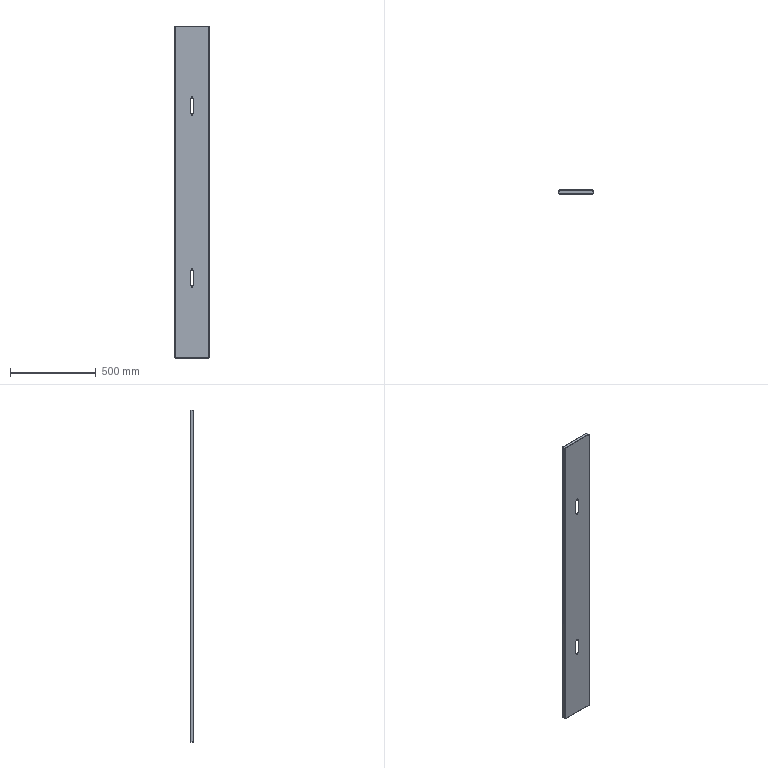Part | STEP file | JBJ-P-1011-07 | 1 solid | 114 faces | box 200 x 20 x 1935 mm | volume 617384 mm3 | plane 58 | cylinder 40 | spline 16 | commonest cylinder face diameters 4 x20 2 x8 4.4 x8 7 x4